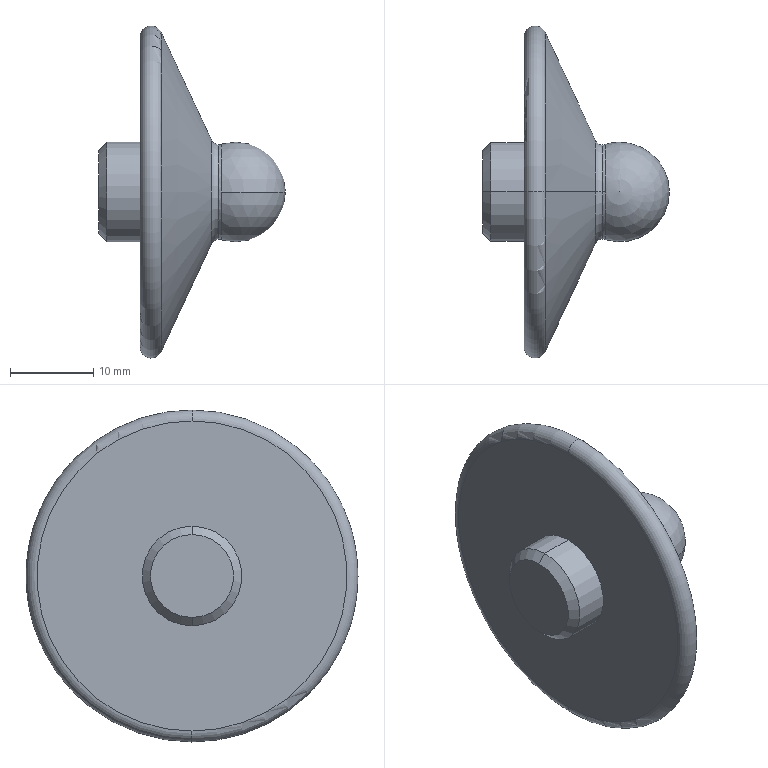Part | SolidWorks | features Chamfer 1, Revolution 1 | 1 solid | 16 faces | box 22.5 x 40 x 40 mm | volume 7773 mm3 | torus 6 | cone 4 | sphere 2 | cylinder 2 | plane 2 | commonest cylinder face diameters 12 x2
STEP:
#1=CARTESIAN_POINT('',(13.572,0.,6.279));
#2=VERTEX_POINT('',#1);
#3=CARTESIAN_POINT('',(14.478,0.,5.702));
#4=VERTEX_POINT('',#3);
#5=CARTESIAN_POINT('',(14.478,0.,6.702));
#6=DIRECTION('',(0.,-1.,0.));
#7=DIRECTION('',(0.,0.,-1.));
#8=AXIS2_PLACEMENT_3D('',#5,#6,#7);
#9=CIRCLE('',#8,1.);
#10=EDGE_CURVE('',#2,#4,#9,.T.);
#11=ORIENTED_EDGE('',*,*,#10,.T.);
#12=CARTESIAN_POINT('',(14.478,0.,-5.702));
#13=VERTEX_POINT('',#12);
#14=CARTESIAN_POINT('',(14.478,0.,0.));
#15=DIRECTION('',(-1.,0.,0.));
#16=DIRECTION('',(0.,0.,1.));
#17=AXIS2_PLACEMENT_3D('',#14,#15,#16);
#18=CIRCLE('',#17,5.702);
#19=EDGE_CURVE('',#4,#13,#18,.T.);
#20=ORIENTED_EDGE('',*,*,#19,.T.);
#21=CARTESIAN_POINT('',(13.572,0.,-6.279));
#22=VERTEX_POINT('',#21);
#23=CARTESIAN_POINT('',(14.478,0.,-6.702));
#24=DIRECTION('',(0.,1.,0.));
#25=DIRECTION('',(0.,0.,1.));
#26=AXIS2_PLACEMENT_3D('',#23,#24,#25);
#27=CIRCLE('',#26,1.);
#28=EDGE_CURVE('',#22,#13,#27,.T.);
#29=ORIENTED_EDGE('',*,*,#28,.F.);
#30=CARTESIAN_POINT('',(13.572,0.,0.));
#31=DIRECTION('',(-1.,0.,0.));
#32=DIRECTION('',(0.,0.,1.));
#33=AXIS2_PLACEMENT_3D('',#30,#31,#32);
#34=CIRCLE('',#33,6.279);
#35=EDGE_CURVE('',#2,#22,#34,.T.);
#36=ORIENTED_EDGE('',*,*,#35,.F.);
#37=EDGE_LOOP('',(#11,#20,#29,#36));
#38=FACE_OUTER_BOUND('',#37,.T.);
#39=CARTESIAN_POINT('',(14.478,0.,0.));
#40=DIRECTION('',(-1.,0.,0.));
#41=DIRECTION('',(0.,0.,1.));
#42=AXIS2_PLACEMENT_3D('',#39,#40,#41);
#43=TOROIDAL_SURFACE('',#42,6.702,1.);
#44=ADVANCED_FACE('',(#38),#43,.F.);
#45=ORIENTED_EDGE('',*,*,#28,.T.);
#46=CARTESIAN_POINT('',(14.478,0.,0.));
#47=DIRECTION('',(-1.,0.,0.));
#48=DIRECTION('',(0.,0.,1.));
#49=AXIS2_PLACEMENT_3D('',#46,#47,#48);
#50=CIRCLE('',#49,5.702);
#51=EDGE_CURVE('',#13,#4,#50,.T.);
#52=ORIENTED_EDGE('',*,*,#51,.T.);
#53=ORIENTED_EDGE('',*,*,#10,.F.);
#54=CARTESIAN_POINT('',(13.572,0.,0.));
#55=DIRECTION('',(-1.,0.,0.));
#56=DIRECTION('',(0.,0.,1.));
#57=AXIS2_PLACEMENT_3D('',#54,#55,#56);
#58=CIRCLE('',#57,6.279);
#59=EDGE_CURVE('',#22,#2,#58,.T.);
#60=ORIENTED_EDGE('',*,*,#59,.F.);
#61=EDGE_LOOP('',(#45,#52,#53,#60));
#62=FACE_OUTER_BOUND('',#61,.T.);
#63=CARTESIAN_POINT('',(14.478,0.,0.));
#64=DIRECTION('',(-1.,0.,0.));
#65=DIRECTION('',(0.,0.,1.));
#66=AXIS2_PLACEMENT_3D('',#63,#64,#65);
#67=TOROIDAL_SURFACE('',#66,6.702,1.);
#68=ADVANCED_FACE('',(#62),#67,.F.);
#69=CARTESIAN_POINT('',(0.,0.,5.));
#70=VERTEX_POINT('',#69);
#71=CARTESIAN_POINT('',(0.,0.,-5.));
#72=VERTEX_POINT('',#71);
#73=CARTESIAN_POINT('',(0.,0.,0.));
#74=DIRECTION('',(-1.,0.,0.));
#75=DIRECTION('',(0.,0.,-1.));
#76=AXIS2_PLACEMENT_3D('',#73,#74,#75);
#77=CIRCLE('',#76,5.);
#78=EDGE_CURVE('',#70,#72,#77,.T.);
#79=ORIENTED_EDGE('',*,*,#78,.F.);
#80=CARTESIAN_POINT('',(1.,0.,6.));
#81=VERTEX_POINT('',#80);
#82=CARTESIAN_POINT('',(0.,0.,5.));
#83=DIRECTION('',(0.7071,0.,0.7071));
#84=VECTOR('',#83,1000.);
#85=LINE('',#82,#84);
#86=EDGE_CURVE('',#70,#81,#85,.T.);
#87=ORIENTED_EDGE('',*,*,#86,.T.);
#88=CARTESIAN_POINT('',(1.,0.,-6.));
#89=VERTEX_POINT('',#88);
#90=CARTESIAN_POINT('',(1.,0.,0.));
#91=DIRECTION('',(1.,0.,0.));
#92=DIRECTION('',(0.,0.,-1.));
#93=AXIS2_PLACEMENT_3D('',#90,#91,#92);
#94=CIRCLE('',#93,6.);
#95=EDGE_CURVE('',#89,#81,#94,.T.);
#96=ORIENTED_EDGE('',*,*,#95,.F.);
#97=CARTESIAN_POINT('',(0.,0.,-5.));
#98=DIRECTION('',(0.7071,0.,-0.7071));
#99=VECTOR('',#98,1000.);
#100=LINE('',#97,#99);
#101=EDGE_CURVE('',#72,#89,#100,.T.);
#102=ORIENTED_EDGE('',*,*,#101,.F.);
#103=EDGE_LOOP('',(#79,#87,#96,#102));
#104=FACE_OUTER_BOUND('',#103,.T.);
#105=CARTESIAN_POINT('',(0.,0.,0.));
#106=DIRECTION('',(1.,0.,0.));
#107=DIRECTION('',(0.,0.,-1.));
#108=AXIS2_PLACEMENT_3D('',#105,#106,#107);
#109=CONICAL_SURFACE('',#108,5.,0.7854);
#110=ADVANCED_FACE('',(#104),#109,.T.);
#111=CARTESIAN_POINT('',(22.5,0.,0.));
#112=VERTEX_POINT('',#111);
#113=CARTESIAN_POINT('',(14.767,5.744,0.));
#114=VERTEX_POINT('',#113);
#115=CARTESIAN_POINT('',(16.5,0.,0.));
#116=DIRECTION('',(0.,0.,1.));
#117=DIRECTION('',(1.,0.,0.));
#118=AXIS2_PLACEMENT_3D('',#115,#116,#117);
#119=CIRCLE('',#118,6.);
#120=EDGE_CURVE('',#112,#114,#119,.T.);
#121=ORIENTED_EDGE('',*,*,#120,.F.);
#122=CARTESIAN_POINT('',(14.767,-5.744,0.));
#123=VERTEX_POINT('',#122);
#124=CARTESIAN_POINT('',(16.5,0.,0.));
#125=DIRECTION('',(0.,0.,-1.));
#126=DIRECTION('',(0.,1.,0.));
#127=AXIS2_PLACEMENT_3D('',#124,#125,#126);
#128=CIRCLE('',#127,6.);
#129=EDGE_CURVE('',#112,#123,#128,.T.);
#130=ORIENTED_EDGE('',*,*,#129,.T.);
#131=CARTESIAN_POINT('',(14.767,0.,-5.744));
#132=VERTEX_POINT('',#131);
#133=CARTESIAN_POINT('',(14.767,0.,0.));
#134=DIRECTION('',(-1.,0.,0.));
#135=DIRECTION('',(0.,0.,1.));
#136=AXIS2_PLACEMENT_3D('',#133,#134,#135);
#137=CIRCLE('',#136,5.744);
#138=EDGE_CURVE('',#132,#123,#137,.T.);
#139=ORIENTED_EDGE('',*,*,#138,.F.);
#140=CARTESIAN_POINT('',(14.767,0.,0.));
#141=DIRECTION('',(-1.,0.,0.));
#142=DIRECTION('',(0.,0.,1.));
#143=AXIS2_PLACEMENT_3D('',#140,#141,#142);
#144=CIRCLE('',#143,5.744);
#145=EDGE_CURVE('',#114,#132,#144,.T.);
#146=ORIENTED_EDGE('',*,*,#145,.F.);
#147=EDGE_LOOP('',(#121,#130,#139,#146));
#148=FACE_OUTER_BOUND('',#147,.T.);
#149=CARTESIAN_POINT('',(16.5,0.,0.));
#150=DIRECTION('',(0.,0.,-1.));
#151=DIRECTION('',(0.,1.,0.));
#152=AXIS2_PLACEMENT_3D('',#149,#150,#151);
#153=SPHERICAL_SURFACE('',#152,6.);
#154=ADVANCED_FACE('',(#148),#153,.T.);
#155=ORIENTED_EDGE('',*,*,#51,.F.);
#156=CARTESIAN_POINT('',(14.478,0.,-6.702));
#157=DIRECTION('',(0.,1.,0.));
#158=DIRECTION('',(0.,0.,1.));
#159=AXIS2_PLACEMENT_3D('',#156,#157,#158);
#160=CIRCLE('',#159,1.);
#161=EDGE_CURVE('',#13,#132,#160,.T.);
#162=ORIENTED_EDGE('',*,*,#161,.T.);
#163=ORIENTED_EDGE('',*,*,#138,.T.);
#164=CARTESIAN_POINT('',(14.767,0.,5.744));
#165=VERTEX_POINT('',#164);
#166=CARTESIAN_POINT('',(14.767,0.,0.));
#167=DIRECTION('',(-1.,0.,0.));
#168=DIRECTION('',(0.,0.,1.));
#169=AXIS2_PLACEMENT_3D('',#166,#167,#168);
#170=CIRCLE('',#169,5.744);
#171=EDGE_CURVE('',#123,#165,#170,.T.);
#172=ORIENTED_EDGE('',*,*,#171,.T.);
#173=CARTESIAN_POINT('',(14.478,0.,6.702));
#174=DIRECTION('',(0.,-1.,0.));
#175=DIRECTION('',(0.,0.,-1.));
#176=AXIS2_PLACEMENT_3D('',#173,#174,#175);
#177=CIRCLE('',#176,1.);
#178=EDGE_CURVE('',#4,#165,#177,.T.);
#179=ORIENTED_EDGE('',*,*,#178,.F.);
#180=EDGE_LOOP('',(#155,#162,#163,#172,#179));
#181=FACE_OUTER_BOUND('',#180,.T.);
#182=CARTESIAN_POINT('',(14.478,0.,0.));
#183=DIRECTION('',(-1.,0.,0.));
#184=DIRECTION('',(0.,0.,1.));
#185=AXIS2_PLACEMENT_3D('',#182,#183,#184);
#186=TOROIDAL_SURFACE('',#185,6.702,1.);
#187=ADVANCED_FACE('',(#181),#186,.F.);
#188=ORIENTED_EDGE('',*,*,#35,.T.);
#189=CARTESIAN_POINT('',(7.531,0.,-19.233));
#190=VERTEX_POINT('',#189);
#191=CARTESIAN_POINT('',(13.572,0.,-6.279));
#192=DIRECTION('',(-0.4226,0.,-0.9063));
#193=VECTOR('',#192,1000.);
#194=LINE('',#191,#193);
#195=EDGE_CURVE('',#22,#190,#194,.T.);
#196=ORIENTED_EDGE('',*,*,#195,.T.);
#197=CARTESIAN_POINT('',(7.531,0.,19.233));
#198=VERTEX_POINT('',#197);
#199=CARTESIAN_POINT('',(7.531,0.,0.));
#200=DIRECTION('',(-1.,0.,0.));
#201=DIRECTION('',(0.,0.,1.));
#202=AXIS2_PLACEMENT_3D('',#199,#200,#201);
#203=CIRCLE('',#202,19.233);
#204=EDGE_CURVE('',#198,#190,#203,.T.);
#205=ORIENTED_EDGE('',*,*,#204,.F.);
#206=CARTESIAN_POINT('',(13.572,0.,6.279));
#207=DIRECTION('',(-0.4226,0.,0.9063));
#208=VECTOR('',#207,1000.);
#209=LINE('',#206,#208);
#210=EDGE_CURVE('',#2,#198,#209,.T.);
#211=ORIENTED_EDGE('',*,*,#210,.F.);
#212=EDGE_LOOP('',(#188,#196,#205,#211));
#213=FACE_OUTER_BOUND('',#212,.T.);
#214=CARTESIAN_POINT('',(13.572,0.,0.));
#215=DIRECTION('',(-1.,0.,0.));
#216=DIRECTION('',(0.,0.,1.));
#217=AXIS2_PLACEMENT_3D('',#214,#215,#216);
#218=CONICAL_SURFACE('',#217,6.279,1.134);
#219=ADVANCED_FACE('',(#213),#218,.T.);
#220=ORIENTED_EDGE('',*,*,#204,.T.);
#221=CARTESIAN_POINT('',(5.,0.,-18.672));
#222=VERTEX_POINT('',#221);
#223=CARTESIAN_POINT('',(6.328,0.,-18.672));
#224=DIRECTION('',(0.,1.,0.));
#225=DIRECTION('',(0.,0.,1.));
#226=AXIS2_PLACEMENT_3D('',#223,#224,#225);
#227=CIRCLE('',#226,1.328);
#228=EDGE_CURVE('',#190,#222,#227,.T.);
#229=ORIENTED_EDGE('',*,*,#228,.T.);
#230=CARTESIAN_POINT('',(5.,0.,18.672));
#231=VERTEX_POINT('',#230);
#232=CARTESIAN_POINT('',(5.,0.,0.));
#233=DIRECTION('',(-1.,0.,0.));
#234=DIRECTION('',(0.,0.,1.));
#235=AXIS2_PLACEMENT_3D('',#232,#233,#234);
#236=CIRCLE('',#235,18.672);
#237=EDGE_CURVE('',#231,#222,#236,.T.);
#238=ORIENTED_EDGE('',*,*,#237,.F.);
#239=CARTESIAN_POINT('',(6.328,0.,18.672));
#240=DIRECTION('',(0.,-1.,0.));
#241=DIRECTION('',(0.,0.,-1.));
#242=AXIS2_PLACEMENT_3D('',#239,#240,#241);
#243=CIRCLE('',#242,1.328);
#244=EDGE_CURVE('',#198,#231,#243,.T.);
#245=ORIENTED_EDGE('',*,*,#244,.F.);
#246=EDGE_LOOP('',(#220,#229,#238,#245));
#247=FACE_OUTER_BOUND('',#246,.T.);
#248=CARTESIAN_POINT('',(6.328,0.,0.));
#249=DIRECTION('',(-1.,0.,0.));
#250=DIRECTION('',(0.,0.,1.));
#251=AXIS2_PLACEMENT_3D('',#248,#249,#250);
#252=TOROIDAL_SURFACE('',#251,18.672,1.328);
#253=ADVANCED_FACE('',(#247),#252,.T.);
#254=CARTESIAN_POINT('',(5.,0.,6.));
#255=VERTEX_POINT('',#254);
#256=CARTESIAN_POINT('',(5.,0.,-6.));
#257=VERTEX_POINT('',#256);
#258=CARTESIAN_POINT('',(5.,0.,0.));
#259=DIRECTION('',(-1.,0.,0.));
#260=DIRECTION('',(0.,0.,1.));
#261=AXIS2_PLACEMENT_3D('',#258,#259,#260);
#262=CIRCLE('',#261,6.);
#263=EDGE_CURVE('',#255,#257,#262,.T.);
#264=ORIENTED_EDGE('',*,*,#263,.T.);
#265=CARTESIAN_POINT('',(0.,0.,-6.));
#266=DIRECTION('',(-1.,0.,0.));
#267=VECTOR('',#266,1000.);
#268=LINE('',#265,#267);
#269=EDGE_CURVE('',#257,#89,#268,.T.);
#270=ORIENTED_EDGE('',*,*,#269,.T.);
#271=ORIENTED_EDGE('',*,*,#95,.T.);
#272=CARTESIAN_POINT('',(0.,0.,6.));
#273=DIRECTION('',(-1.,0.,0.));
#274=VECTOR('',#273,1000.);
#275=LINE('',#272,#274);
#276=EDGE_CURVE('',#255,#81,#275,.T.);
#277=ORIENTED_EDGE('',*,*,#276,.F.);
#278=EDGE_LOOP('',(#264,#270,#271,#277));
#279=FACE_OUTER_BOUND('',#278,.T.);
#280=CARTESIAN_POINT('',(0.,0.,0.));
#281=DIRECTION('',(-1.,0.,0.));
#282=DIRECTION('',(0.,0.,1.));
#283=AXIS2_PLACEMENT_3D('',#280,#281,#282);
#284=CYLINDRICAL_SURFACE('',#283,6.);
#285=ADVANCED_FACE('',(#279),#284,.T.);
#286=CARTESIAN_POINT('',(0.,0.,0.));
#287=DIRECTION('',(-1.,0.,0.));
#288=DIRECTION('',(0.,0.,-1.));
#289=AXIS2_PLACEMENT_3D('',#286,#287,#288);
#290=CIRCLE('',#289,5.);
#291=EDGE_CURVE('',#72,#70,#290,.T.);
#292=ORIENTED_EDGE('',*,*,#291,.T.);
#293=ORIENTED_EDGE('',*,*,#78,.T.);
#294=EDGE_LOOP('',(#292,#293));
#295=FACE_OUTER_BOUND('',#294,.T.);
#296=CARTESIAN_POINT('',(0.,0.,0.));
#297=DIRECTION('',(1.,0.,0.));
#298=DIRECTION('',(0.,0.,-1.));
#299=AXIS2_PLACEMENT_3D('',#296,#297,#298);
#300=PLANE('',#299);
#301=ADVANCED_FACE('',(#295),#300,.F.);
#302=ORIENTED_EDGE('',*,*,#269,.F.);
#303=CARTESIAN_POINT('',(5.,0.,0.));
#304=DIRECTION('',(-1.,0.,0.));
#305=DIRECTION('',(0.,0.,1.));
#306=AXIS2_PLACEMENT_3D('',#303,#304,#305);
#307=CIRCLE('',#306,6.);
#308=EDGE_CURVE('',#257,#255,#307,.T.);
#309=ORIENTED_EDGE('',*,*,#308,.T.);
#310=ORIENTED_EDGE('',*,*,#276,.T.);
#311=CARTESIAN_POINT('',(1.,0.,0.));
#312=DIRECTION('',(1.,0.,0.));
#313=DIRECTION('',(0.,0.,-1.));
#314=AXIS2_PLACEMENT_3D('',#311,#312,#313);
#315=CIRCLE('',#314,6.);
#316=EDGE_CURVE('',#81,#89,#315,.T.);
#317=ORIENTED_EDGE('',*,*,#316,.T.);
#318=EDGE_LOOP('',(#302,#309,#310,#317));
#319=FACE_OUTER_BOUND('',#318,.T.);
#320=CARTESIAN_POINT('',(0.,0.,0.));
#321=DIRECTION('',(-1.,0.,0.));
#322=DIRECTION('',(0.,0.,1.));
#323=AXIS2_PLACEMENT_3D('',#320,#321,#322);
#324=CYLINDRICAL_SURFACE('',#323,6.);
#325=ADVANCED_FACE('',(#319),#324,.T.);
#326=ORIENTED_EDGE('',*,*,#263,.F.);
#327=ORIENTED_EDGE('',*,*,#308,.F.);
#328=EDGE_LOOP('',(#326,#327));
#329=FACE_BOUND('',#328,.T.);
#330=ORIENTED_EDGE('',*,*,#237,.T.);
#331=CARTESIAN_POINT('',(5.,0.,0.));
#332=DIRECTION('',(-1.,0.,0.));
#333=DIRECTION('',(0.,0.,1.));
#334=AXIS2_PLACEMENT_3D('',#331,#332,#333);
#335=CIRCLE('',#334,18.672);
#336=EDGE_CURVE('',#222,#231,#335,.T.);
#337=ORIENTED_EDGE('',*,*,#336,.T.);
#338=EDGE_LOOP('',(#330,#337));
#339=FACE_OUTER_BOUND('',#338,.T.);
#340=CARTESIAN_POINT('',(5.,6.,0.));
#341=DIRECTION('',(1.,0.,0.));
#342=DIRECTION('',(0.,0.,-1.));
#343=AXIS2_PLACEMENT_3D('',#340,#341,#342);
#344=PLANE('',#343);
#345=ADVANCED_FACE('',(#329,#339),#344,.F.);
#346=ORIENTED_EDGE('',*,*,#228,.F.);
#347=CARTESIAN_POINT('',(7.531,0.,0.));
#348=DIRECTION('',(-1.,0.,0.));
#349=DIRECTION('',(0.,0.,1.));
#350=AXIS2_PLACEMENT_3D('',#347,#348,#349);
#351=CIRCLE('',#350,19.233);
#352=EDGE_CURVE('',#190,#198,#351,.T.);
#353=ORIENTED_EDGE('',*,*,#352,.T.);
#354=ORIENTED_EDGE('',*,*,#244,.T.);
#355=ORIENTED_EDGE('',*,*,#336,.F.);
#356=EDGE_LOOP('',(#346,#353,#354,#355));
#357=FACE_OUTER_BOUND('',#356,.T.);
#358=CARTESIAN_POINT('',(6.328,0.,0.));
#359=DIRECTION('',(-1.,0.,0.));
#360=DIRECTION('',(0.,0.,1.));
#361=AXIS2_PLACEMENT_3D('',#358,#359,#360);
#362=TOROIDAL_SURFACE('',#361,18.672,1.328);
#363=ADVANCED_FACE('',(#357),#362,.T.);
#364=ORIENTED_EDGE('',*,*,#195,.F.);
#365=ORIENTED_EDGE('',*,*,#59,.T.);
#366=ORIENTED_EDGE('',*,*,#210,.T.);
#367=ORIENTED_EDGE('',*,*,#352,.F.);
#368=EDGE_LOOP('',(#364,#365,#366,#367));
#369=FACE_OUTER_BOUND('',#368,.T.);
#370=CARTESIAN_POINT('',(13.572,0.,0.));
#371=DIRECTION('',(-1.,0.,0.));
#372=DIRECTION('',(0.,0.,1.));
#373=AXIS2_PLACEMENT_3D('',#370,#371,#372);
#374=CONICAL_SURFACE('',#373,6.279,1.134);
#375=ADVANCED_FACE('',(#369),#374,.T.);
#376=ORIENTED_EDGE('',*,*,#19,.F.);
#377=ORIENTED_EDGE('',*,*,#178,.T.);
#378=CARTESIAN_POINT('',(14.767,0.,0.));
#379=DIRECTION('',(-1.,0.,0.));
#380=DIRECTION('',(0.,0.,1.));
#381=AXIS2_PLACEMENT_3D('',#378,#379,#380);
#382=CIRCLE('',#381,5.744);
#383=EDGE_CURVE('',#165,#114,#382,.T.);
#384=ORIENTED_EDGE('',*,*,#383,.T.);
#385=ORIENTED_EDGE('',*,*,#145,.T.);
#386=ORIENTED_EDGE('',*,*,#161,.F.);
#387=EDGE_LOOP('',(#376,#377,#384,#385,#386));
#388=FACE_OUTER_BOUND('',#387,.T.);
#389=CARTESIAN_POINT('',(14.478,0.,0.));
#390=DIRECTION('',(-1.,0.,0.));
#391=DIRECTION('',(0.,0.,1.));
#392=AXIS2_PLACEMENT_3D('',#389,#390,#391);
#393=TOROIDAL_SURFACE('',#392,6.702,1.);
#394=ADVANCED_FACE('',(#388),#393,.F.);
#395=ORIENTED_EDGE('',*,*,#129,.F.);
#396=ORIENTED_EDGE('',*,*,#120,.T.);
#397=ORIENTED_EDGE('',*,*,#383,.F.);
#398=ORIENTED_EDGE('',*,*,#171,.F.);
#399=EDGE_LOOP('',(#395,#396,#397,#398));
#400=FACE_OUTER_BOUND('',#399,.T.);
#401=CARTESIAN_POINT('',(16.5,0.,0.));
#402=DIRECTION('',(0.,0.,-1.));
#403=DIRECTION('',(0.,1.,0.));
#404=AXIS2_PLACEMENT_3D('',#401,#402,#403);
#405=SPHERICAL_SURFACE('',#404,6.);
#406=ADVANCED_FACE('',(#400),#405,.T.);
#407=ORIENTED_EDGE('',*,*,#86,.F.);
#408=ORIENTED_EDGE('',*,*,#291,.F.);
#409=ORIENTED_EDGE('',*,*,#101,.T.);
#410=ORIENTED_EDGE('',*,*,#316,.F.);
#411=EDGE_LOOP('',(#407,#408,#409,#410));
#412=FACE_OUTER_BOUND('',#411,.T.);
#413=CARTESIAN_POINT('',(0.,0.,0.));
#414=DIRECTION('',(1.,0.,0.));
#415=DIRECTION('',(0.,0.,-1.));
#416=AXIS2_PLACEMENT_3D('',#413,#414,#415);
#417=CONICAL_SURFACE('',#416,5.,0.7854);
#418=ADVANCED_FACE('',(#412),#417,.T.);
#419=CLOSED_SHELL('',(#44,#68,#110,#154,#187,#219,#253,#285,#301,#325,#345,#363,#375,#394,#406,#418));
#420=MANIFOLD_SOLID_BREP('',#419);
#421=CARTESIAN_POINT('',(0.,0.,0.));
#422=DIRECTION('',(0.,0.,1.));
#423=DIRECTION('',(1.,0.,0.));
#424=AXIS2_PLACEMENT_3D('',#421,#422,#423);
#425=(LENGTH_UNIT()NAMED_UNIT(*)SI_UNIT(.MILLI.,.METRE.));
#426=UNCERTAINTY_MEASURE_WITH_UNIT(LENGTH_MEASURE(0.00001),#425,'','');
#427=(NAMED_UNIT(*)PLANE_ANGLE_UNIT()SI_UNIT($,.RADIAN.));
#428=(NAMED_UNIT(*)SI_UNIT($,.STERADIAN.)SOLID_ANGLE_UNIT());
#429=(GEOMETRIC_REPRESENTATION_CONTEXT(3)GLOBAL_UNCERTAINTY_ASSIGNED_CONTEXT((#426))GLOBAL_UNIT_ASSIGNED_CONTEXT((#425,#427,#428))REPRESENTATION_CONTEXT('',''));
#430=ADVANCED_BREP_SHAPE_REPRESENTATION('',(#420,#424),#429);